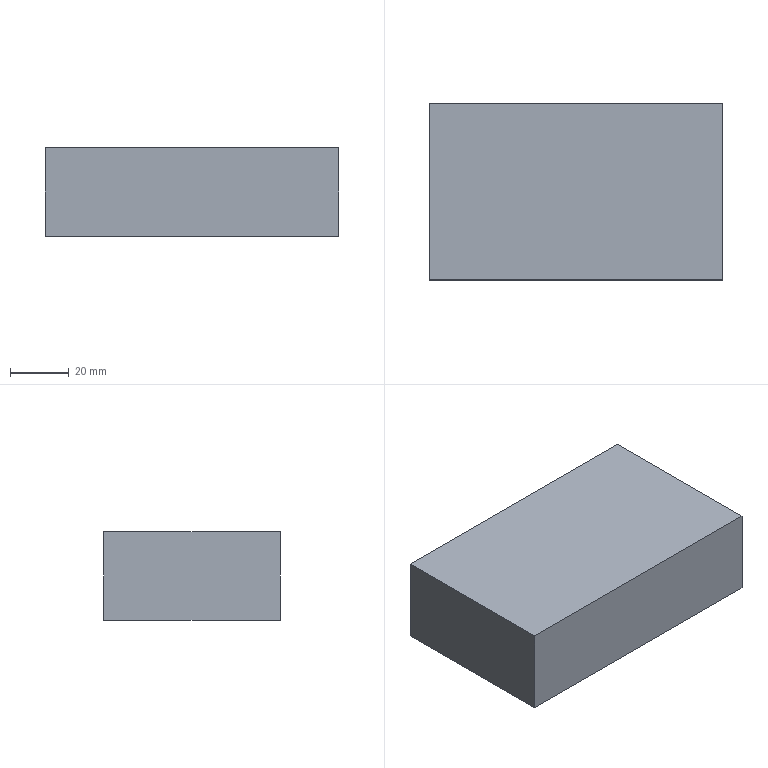Part | SolidWorks | features Extrusion 1 | 1 solid | 6 faces | box 100 x 60 x 30 mm | volume 180000 mm3 | plane 6
STEP:
#1=CARTESIAN_POINT('',(-50.,30.,0.));
#2=VERTEX_POINT('',#1);
#3=CARTESIAN_POINT('',(-50.,-30.,0.));
#4=VERTEX_POINT('',#3);
#5=CARTESIAN_POINT('',(-50.,-30.,0.));
#6=DIRECTION('',(0.,-1.,0.));
#7=VECTOR('',#6,1000.);
#8=LINE('',#5,#7);
#9=EDGE_CURVE('',#2,#4,#8,.T.);
#10=ORIENTED_EDGE('',*,*,#9,.T.);
#11=CARTESIAN_POINT('',(-50.,-30.,30.));
#12=VERTEX_POINT('',#11);
#13=CARTESIAN_POINT('',(-50.,-30.,30.));
#14=DIRECTION('',(0.,0.,-1.));
#15=VECTOR('',#14,1000.);
#16=LINE('',#13,#15);
#17=EDGE_CURVE('',#12,#4,#16,.T.);
#18=ORIENTED_EDGE('',*,*,#17,.F.);
#19=CARTESIAN_POINT('',(-50.,30.,30.));
#20=VERTEX_POINT('',#19);
#21=CARTESIAN_POINT('',(-50.,-30.,30.));
#22=DIRECTION('',(0.,-1.,0.));
#23=VECTOR('',#22,1000.);
#24=LINE('',#21,#23);
#25=EDGE_CURVE('',#20,#12,#24,.T.);
#26=ORIENTED_EDGE('',*,*,#25,.F.);
#27=CARTESIAN_POINT('',(-50.,30.,30.));
#28=DIRECTION('',(0.,0.,-1.));
#29=VECTOR('',#28,1000.);
#30=LINE('',#27,#29);
#31=EDGE_CURVE('',#20,#2,#30,.T.);
#32=ORIENTED_EDGE('',*,*,#31,.T.);
#33=EDGE_LOOP('',(#10,#18,#26,#32));
#34=FACE_OUTER_BOUND('',#33,.T.);
#35=CARTESIAN_POINT('',(-50.,-30.,30.));
#36=DIRECTION('',(1.,0.,0.));
#37=DIRECTION('',(0.,0.,-1.));
#38=AXIS2_PLACEMENT_3D('',#35,#36,#37);
#39=PLANE('',#38);
#40=ADVANCED_FACE('',(#34),#39,.F.);
#41=CARTESIAN_POINT('',(50.,-30.,0.));
#42=VERTEX_POINT('',#41);
#43=CARTESIAN_POINT('',(50.,-30.,0.));
#44=DIRECTION('',(1.,0.,0.));
#45=VECTOR('',#44,1000.);
#46=LINE('',#43,#45);
#47=EDGE_CURVE('',#4,#42,#46,.T.);
#48=ORIENTED_EDGE('',*,*,#47,.T.);
#49=CARTESIAN_POINT('',(50.,-30.,30.));
#50=VERTEX_POINT('',#49);
#51=CARTESIAN_POINT('',(50.,-30.,30.));
#52=DIRECTION('',(0.,0.,-1.));
#53=VECTOR('',#52,1000.);
#54=LINE('',#51,#53);
#55=EDGE_CURVE('',#50,#42,#54,.T.);
#56=ORIENTED_EDGE('',*,*,#55,.F.);
#57=CARTESIAN_POINT('',(50.,-30.,30.));
#58=DIRECTION('',(1.,0.,0.));
#59=VECTOR('',#58,1000.);
#60=LINE('',#57,#59);
#61=EDGE_CURVE('',#12,#50,#60,.T.);
#62=ORIENTED_EDGE('',*,*,#61,.F.);
#63=ORIENTED_EDGE('',*,*,#17,.T.);
#64=EDGE_LOOP('',(#48,#56,#62,#63));
#65=FACE_OUTER_BOUND('',#64,.T.);
#66=CARTESIAN_POINT('',(50.,-30.,30.));
#67=DIRECTION('',(0.,1.,0.));
#68=DIRECTION('',(-1.,0.,0.));
#69=AXIS2_PLACEMENT_3D('',#66,#67,#68);
#70=PLANE('',#69);
#71=ADVANCED_FACE('',(#65),#70,.F.);
#72=CARTESIAN_POINT('',(50.,30.,0.));
#73=VERTEX_POINT('',#72);
#74=CARTESIAN_POINT('',(50.,-30.,0.));
#75=DIRECTION('',(0.,1.,0.));
#76=VECTOR('',#75,1000.);
#77=LINE('',#74,#76);
#78=EDGE_CURVE('',#42,#73,#77,.T.);
#79=ORIENTED_EDGE('',*,*,#78,.T.);
#80=CARTESIAN_POINT('',(50.,30.,30.));
#81=VERTEX_POINT('',#80);
#82=CARTESIAN_POINT('',(50.,30.,30.));
#83=DIRECTION('',(0.,0.,-1.));
#84=VECTOR('',#83,1000.);
#85=LINE('',#82,#84);
#86=EDGE_CURVE('',#81,#73,#85,.T.);
#87=ORIENTED_EDGE('',*,*,#86,.F.);
#88=CARTESIAN_POINT('',(50.,-30.,30.));
#89=DIRECTION('',(0.,1.,0.));
#90=VECTOR('',#89,1000.);
#91=LINE('',#88,#90);
#92=EDGE_CURVE('',#50,#81,#91,.T.);
#93=ORIENTED_EDGE('',*,*,#92,.F.);
#94=ORIENTED_EDGE('',*,*,#55,.T.);
#95=EDGE_LOOP('',(#79,#87,#93,#94));
#96=FACE_OUTER_BOUND('',#95,.T.);
#97=CARTESIAN_POINT('',(50.,-30.,30.));
#98=DIRECTION('',(-1.,0.,0.));
#99=DIRECTION('',(0.,0.,1.));
#100=AXIS2_PLACEMENT_3D('',#97,#98,#99);
#101=PLANE('',#100);
#102=ADVANCED_FACE('',(#96),#101,.F.);
#103=CARTESIAN_POINT('',(50.,30.,0.));
#104=DIRECTION('',(-1.,0.,0.));
#105=VECTOR('',#104,1000.);
#106=LINE('',#103,#105);
#107=EDGE_CURVE('',#73,#2,#106,.T.);
#108=ORIENTED_EDGE('',*,*,#107,.T.);
#109=ORIENTED_EDGE('',*,*,#31,.F.);
#110=CARTESIAN_POINT('',(50.,30.,30.));
#111=DIRECTION('',(-1.,0.,0.));
#112=VECTOR('',#111,1000.);
#113=LINE('',#110,#112);
#114=EDGE_CURVE('',#81,#20,#113,.T.);
#115=ORIENTED_EDGE('',*,*,#114,.F.);
#116=ORIENTED_EDGE('',*,*,#86,.T.);
#117=EDGE_LOOP('',(#108,#109,#115,#116));
#118=FACE_OUTER_BOUND('',#117,.T.);
#119=CARTESIAN_POINT('',(50.,30.,30.));
#120=DIRECTION('',(0.,-1.,0.));
#121=DIRECTION('',(1.,0.,0.));
#122=AXIS2_PLACEMENT_3D('',#119,#120,#121);
#123=PLANE('',#122);
#124=ADVANCED_FACE('',(#118),#123,.F.);
#125=ORIENTED_EDGE('',*,*,#25,.T.);
#126=ORIENTED_EDGE('',*,*,#61,.T.);
#127=ORIENTED_EDGE('',*,*,#92,.T.);
#128=ORIENTED_EDGE('',*,*,#114,.T.);
#129=EDGE_LOOP('',(#125,#126,#127,#128));
#130=FACE_OUTER_BOUND('',#129,.T.);
#131=CARTESIAN_POINT('',(0.,0.,30.));
#132=DIRECTION('',(0.,0.,1.));
#133=DIRECTION('',(1.,0.,0.));
#134=AXIS2_PLACEMENT_3D('',#131,#132,#133);
#135=PLANE('',#134);
#136=ADVANCED_FACE('',(#130),#135,.T.);
#137=ORIENTED_EDGE('',*,*,#9,.F.);
#138=ORIENTED_EDGE('',*,*,#107,.F.);
#139=ORIENTED_EDGE('',*,*,#78,.F.);
#140=ORIENTED_EDGE('',*,*,#47,.F.);
#141=EDGE_LOOP('',(#137,#138,#139,#140));
#142=FACE_OUTER_BOUND('',#141,.T.);
#143=CARTESIAN_POINT('',(0.,0.,0.));
#144=DIRECTION('',(0.,0.,1.));
#145=DIRECTION('',(1.,0.,0.));
#146=AXIS2_PLACEMENT_3D('',#143,#144,#145);
#147=PLANE('',#146);
#148=ADVANCED_FACE('',(#142),#147,.F.);
#149=CLOSED_SHELL('',(#40,#71,#102,#124,#136,#148));
#150=MANIFOLD_SOLID_BREP('',#149);
#151=CARTESIAN_POINT('',(0.,0.,0.));
#152=DIRECTION('',(0.,0.,1.));
#153=DIRECTION('',(1.,0.,0.));
#154=AXIS2_PLACEMENT_3D('',#151,#152,#153);
#155=(LENGTH_UNIT()NAMED_UNIT(*)SI_UNIT(.MILLI.,.METRE.));
#156=UNCERTAINTY_MEASURE_WITH_UNIT(LENGTH_MEASURE(0.00001),#155,'','');
#157=(NAMED_UNIT(*)PLANE_ANGLE_UNIT()SI_UNIT($,.RADIAN.));
#158=(NAMED_UNIT(*)SI_UNIT($,.STERADIAN.)SOLID_ANGLE_UNIT());
#159=(GEOMETRIC_REPRESENTATION_CONTEXT(3)GLOBAL_UNCERTAINTY_ASSIGNED_CONTEXT((#156))GLOBAL_UNIT_ASSIGNED_CONTEXT((#155,#157,#158))REPRESENTATION_CONTEXT('',''));
#160=ADVANCED_BREP_SHAPE_REPRESENTATION('',(#150,#154),#159);